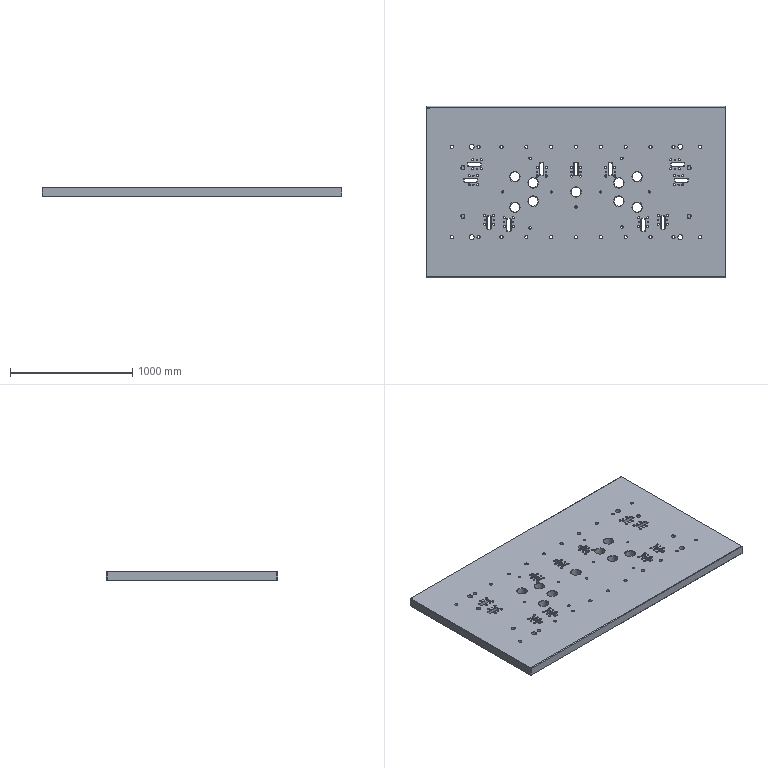Part | STEP file | solid 15 | 1 solid | 498 faces | box 2450 x 1400 x 75.5 mm | volume 249798342 mm3 | plane 198 | cylinder 190 | cone 110 | commonest cylinder face diameters 14 x44 18 x44 26 x26 10 x22 39 x22 80 x9